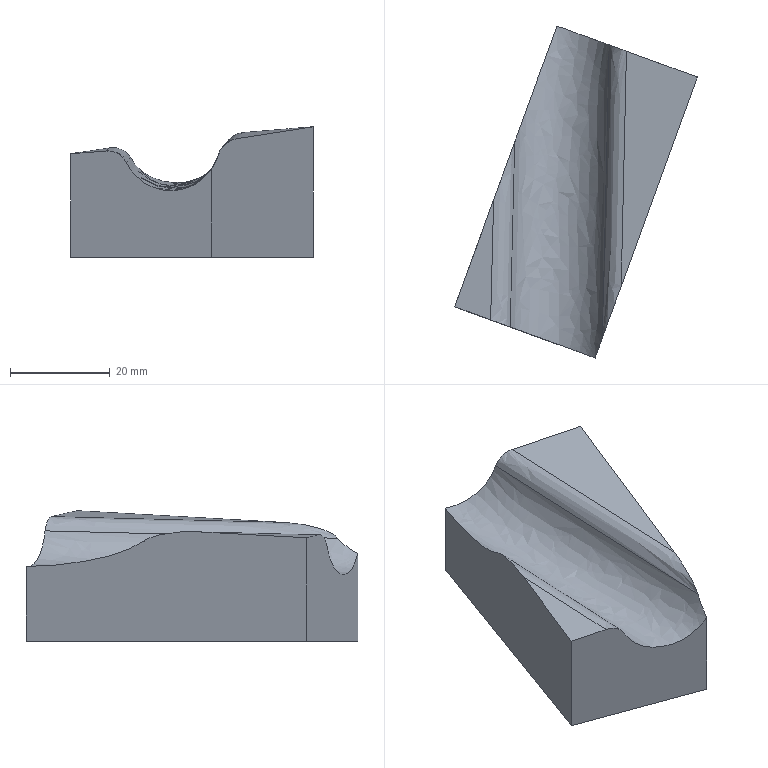Part | NX | features solid 2 | 1 solid | 10 faces | box 48.712 x 66.642 x 26.219 mm | volume 34058 mm3 | plane 5 | spline 5
STEP:
#1=CARTESIAN_POINT('',(673.941,90.778,15.));
#2=VERTEX_POINT('',#1);
#3=CARTESIAN_POINT('',(702.132,80.518,15.));
#4=VERTEX_POINT('',#3);
#5=CARTESIAN_POINT('',(673.941,90.778,15.));
#6=DIRECTION('',(-0.9397,0.342,0.));
#7=VECTOR('',#6,1000.);
#8=LINE('',#5,#7);
#9=EDGE_CURVE('',#2,#4,#8,.F.);
#10=ORIENTED_EDGE('',*,*,#9,.F.);
#11=CARTESIAN_POINT('',(694.463,147.16,15.));
#12=VERTEX_POINT('',#11);
#13=CARTESIAN_POINT('',(694.463,147.16,15.));
#14=DIRECTION('',(0.342,0.9397,0.));
#15=VECTOR('',#14,1000.);
#16=LINE('',#13,#15);
#17=EDGE_CURVE('',#12,#2,#16,.F.);
#18=ORIENTED_EDGE('',*,*,#17,.F.);
#19=CARTESIAN_POINT('',(722.653,136.899,15.));
#20=VERTEX_POINT('',#19);
#21=CARTESIAN_POINT('',(694.463,147.16,15.));
#22=DIRECTION('',(0.9397,-0.342,0.));
#23=VECTOR('',#22,1000.);
#24=LINE('',#21,#23);
#25=EDGE_CURVE('',#12,#20,#24,.T.);
#26=ORIENTED_EDGE('',*,*,#25,.T.);
#27=CARTESIAN_POINT('',(722.653,136.899,15.));
#28=DIRECTION('',(-0.342,-0.9397,0.));
#29=VECTOR('',#28,1000.);
#30=LINE('',#27,#29);
#31=EDGE_CURVE('',#20,#4,#30,.T.);
#32=ORIENTED_EDGE('',*,*,#31,.T.);
#33=EDGE_LOOP('',(#10,#18,#26,#32));
#34=FACE_BOUND('',#33,.T.);
#35=CARTESIAN_POINT('',(694.463,147.16,15.));
#36=DIRECTION('',(0.,0.,-1.));
#37=DIRECTION('',(-1.,0.,0.));
#38=AXIS2_PLACEMENT_3D('',#35,#36,#37);
#39=PLANE('',#38);
#40=ADVANCED_FACE('',(#34),#39,.T.);
#41=CARTESIAN_POINT('',(707.372,94.917,38.833));
#42=VERTEX_POINT('',#41);
#43=CARTESIAN_POINT('',(722.653,136.899,41.219));
#44=VERTEX_POINT('',#43);
#45=CARTESIAN_POINT('',(707.373,94.917,38.833));
#46=CARTESIAN_POINT('',(712.467,108.911,39.622));
#47=CARTESIAN_POINT('',(717.56,122.905,40.417));
#48=CARTESIAN_POINT('',(722.653,136.899,41.219));
#49=B_SPLINE_CURVE_WITH_KNOTS('',3,(#45,#46,#47,#48),.UNSPECIFIED.,.F.,.F.,(4,4),(0.01534,0.06009),.UNSPECIFIED.);
#50=EDGE_CURVE('',#42,#44,#49,.T.);
#51=ORIENTED_EDGE('',*,*,#50,.F.);
#52=CARTESIAN_POINT('',(703.614,84.589,35.684));
#53=VERTEX_POINT('',#52);
#54=CARTESIAN_POINT('',(707.373,94.917,38.833));
#55=CARTESIAN_POINT('',(707.041,94.005,38.782));
#56=CARTESIAN_POINT('',(706.382,92.195,38.607));
#57=CARTESIAN_POINT('',(705.407,89.515,38.119));
#58=CARTESIAN_POINT('',(704.453,86.895,37.295));
#59=CARTESIAN_POINT('',(703.838,85.206,36.423));
#60=CARTESIAN_POINT('',(703.614,84.59,35.686));
#61=B_SPLINE_CURVE_WITH_KNOTS('',3,(#54,#55,#56,#57,#58,#59,#60),.UNSPECIFIED.,.F.,.F.,(4,1,1,1,4),(0.,0.002892,0.005784,0.008676,0.01157),.UNSPECIFIED.);
#62=EDGE_CURVE('',#42,#53,#61,.T.);
#63=ORIENTED_EDGE('',*,*,#62,.T.);
#64=CARTESIAN_POINT('',(702.132,80.518,32.614));
#65=VERTEX_POINT('',#64);
#66=CARTESIAN_POINT('',(703.613,84.588,35.683));
#67=CARTESIAN_POINT('',(703.208,83.472,34.348));
#68=CARTESIAN_POINT('',(702.681,82.026,33.406));
#69=CARTESIAN_POINT('',(702.132,80.518,32.614));
#70=B_SPLINE_CURVE_WITH_KNOTS('',3,(#66,#67,#68,#69),.UNSPECIFIED.,.F.,.F.,(4,4),(0.0005394,0.005844),.UNSPECIFIED.);
#71=EDGE_CURVE('',#53,#65,#70,.T.);
#72=ORIENTED_EDGE('',*,*,#71,.T.);
#73=CARTESIAN_POINT('',(702.132,80.518,13.));
#74=DIRECTION('',(0.,0.,1.));
#75=VECTOR('',#74,1000.);
#76=LINE('',#73,#75);
#77=EDGE_CURVE('',#4,#65,#76,.T.);
#78=ORIENTED_EDGE('',*,*,#77,.F.);
#79=ORIENTED_EDGE('',*,*,#31,.F.);
#80=CARTESIAN_POINT('',(722.653,136.899,13.));
#81=DIRECTION('',(0.,0.,1.));
#82=VECTOR('',#81,1000.);
#83=LINE('',#80,#82);
#84=EDGE_CURVE('',#20,#44,#83,.T.);
#85=ORIENTED_EDGE('',*,*,#84,.T.);
#86=EDGE_LOOP('',(#51,#63,#72,#78,#79,#85));
#87=FACE_BOUND('',#86,.T.);
#88=CARTESIAN_POINT('',(722.653,136.899,13.));
#89=DIRECTION('',(0.9397,-0.342,0.));
#90=DIRECTION('',(-0.342,-0.9397,0.));
#91=AXIS2_PLACEMENT_3D('',#88,#89,#90);
#92=PLANE('',#91);
#93=ADVANCED_FACE('',(#87),#92,.T.);
#94=CARTESIAN_POINT('',(673.941,90.778,35.787));
#95=VERTEX_POINT('',#94);
#96=CARTESIAN_POINT('',(681.155,88.153,36.347));
#97=VERTEX_POINT('',#96);
#98=CARTESIAN_POINT('',(673.941,90.778,35.787));
#99=CARTESIAN_POINT('',(676.346,89.903,35.972));
#100=CARTESIAN_POINT('',(678.75,89.028,36.159));
#101=CARTESIAN_POINT('',(681.155,88.153,36.347));
#102=B_SPLINE_CURVE_WITH_KNOTS('',3,(#98,#99,#100,#101),.UNSPECIFIED.,.F.,.F.,(4,4),(0.,0.007697),.UNSPECIFIED.);
#103=EDGE_CURVE('',#95,#97,#102,.T.);
#104=ORIENTED_EDGE('',*,*,#103,.F.);
#105=CARTESIAN_POINT('',(673.941,90.778,13.));
#106=DIRECTION('',(0.,0.,1.));
#107=VECTOR('',#106,1000.);
#108=LINE('',#105,#107);
#109=EDGE_CURVE('',#2,#95,#108,.T.);
#110=ORIENTED_EDGE('',*,*,#109,.F.);
#111=ORIENTED_EDGE('',*,*,#9,.T.);
#112=ORIENTED_EDGE('',*,*,#77,.T.);
#113=CARTESIAN_POINT('',(685.071,86.728,34.051));
#114=VERTEX_POINT('',#113);
#115=CARTESIAN_POINT('',(702.132,80.518,32.614));
#116=CARTESIAN_POINT('',(700.144,81.242,29.648));
#117=CARTESIAN_POINT('',(693.105,83.803,26.583));
#118=CARTESIAN_POINT('',(686.604,86.17,30.796));
#119=CARTESIAN_POINT('',(685.071,86.728,34.051));
#120=B_SPLINE_CURVE_WITH_KNOTS('',3,(#115,#116,#117,#118,#119),.UNSPECIFIED.,.F.,.F.,(4,1,4),(0.,0.01075,0.0215),.UNSPECIFIED.);
#121=EDGE_CURVE('',#65,#114,#120,.T.);
#122=ORIENTED_EDGE('',*,*,#121,.T.);
#123=CARTESIAN_POINT('',(685.071,86.728,34.051));
#124=CARTESIAN_POINT('',(684.357,86.988,35.567));
#125=CARTESIAN_POINT('',(682.743,87.575,36.471));
#126=CARTESIAN_POINT('',(681.156,88.153,36.347));
#127=B_SPLINE_CURVE_WITH_KNOTS('',3,(#123,#124,#125,#126),.UNSPECIFIED.,.F.,.F.,(4,4),(0.,0.005011),.UNSPECIFIED.);
#128=EDGE_CURVE('',#114,#97,#127,.T.);
#129=ORIENTED_EDGE('',*,*,#128,.T.);
#130=EDGE_LOOP('',(#104,#110,#111,#112,#122,#129));
#131=FACE_BOUND('',#130,.T.);
#132=CARTESIAN_POINT('',(673.941,90.778,13.));
#133=DIRECTION('',(0.342,0.9397,0.));
#134=DIRECTION('',(0.9397,-0.342,0.));
#135=AXIS2_PLACEMENT_3D('',#132,#133,#134);
#136=PLANE('',#135);
#137=ADVANCED_FACE('',(#131),#136,.F.);
#138=CARTESIAN_POINT('',(681.758,112.256,36.959));
#139=VERTEX_POINT('',#138);
#140=CARTESIAN_POINT('',(681.758,112.256,36.959));
#141=CARTESIAN_POINT('',(679.153,105.097,36.567));
#142=CARTESIAN_POINT('',(676.547,97.938,36.176));
#143=CARTESIAN_POINT('',(673.941,90.778,35.787));
#144=B_SPLINE_CURVE_WITH_KNOTS('',3,(#140,#141,#142,#143),.UNSPECIFIED.,.F.,.F.,(4,4),(0.03719,0.06008),.UNSPECIFIED.);
#145=EDGE_CURVE('',#139,#95,#144,.T.);
#146=ORIENTED_EDGE('',*,*,#145,.F.);
#147=CARTESIAN_POINT('',(685.973,123.834,34.991));
#148=VERTEX_POINT('',#147);
#149=CARTESIAN_POINT('',(681.758,112.256,36.959));
#150=CARTESIAN_POINT('',(682.48,114.238,37.067));
#151=CARTESIAN_POINT('',(683.556,117.194,37.));
#152=CARTESIAN_POINT('',(684.984,121.118,36.247));
#153=CARTESIAN_POINT('',(685.663,122.984,35.579));
#154=CARTESIAN_POINT('',(685.973,123.834,34.991));
#155=B_SPLINE_CURVE_WITH_KNOTS('',3,(#149,#150,#151,#152,#153,#154),.UNSPECIFIED.,.F.,.F.,(4,1,1,4),(0.,0.006299,0.009448,0.0126),.UNSPECIFIED.);
#156=EDGE_CURVE('',#139,#148,#155,.T.);
#157=ORIENTED_EDGE('',*,*,#156,.T.);
#158=CARTESIAN_POINT('',(694.463,147.16,30.025));
#159=VERTEX_POINT('',#158);
#160=CARTESIAN_POINT('',(685.973,123.834,34.991));
#161=CARTESIAN_POINT('',(686.592,125.535,33.816));
#162=CARTESIAN_POINT('',(687.975,129.336,32.282));
#163=CARTESIAN_POINT('',(690.829,137.177,30.562));
#164=CARTESIAN_POINT('',(693.001,143.144,30.075));
#165=CARTESIAN_POINT('',(694.463,147.16,30.025));
#166=B_SPLINE_CURVE_WITH_KNOTS('',3,(#160,#161,#162,#163,#164,#165),.UNSPECIFIED.,.F.,.F.,(4,1,1,4),(0.000493,0.006904,0.01332,0.02614),.UNSPECIFIED.);
#167=EDGE_CURVE('',#148,#159,#166,.T.);
#168=ORIENTED_EDGE('',*,*,#167,.T.);
#169=CARTESIAN_POINT('',(694.463,147.16,13.));
#170=DIRECTION('',(0.,0.,1.));
#171=VECTOR('',#170,1000.);
#172=LINE('',#169,#171);
#173=EDGE_CURVE('',#12,#159,#172,.T.);
#174=ORIENTED_EDGE('',*,*,#173,.F.);
#175=ORIENTED_EDGE('',*,*,#17,.T.);
#176=ORIENTED_EDGE('',*,*,#109,.T.);
#177=EDGE_LOOP('',(#146,#157,#168,#174,#175,#176));
#178=FACE_BOUND('',#177,.T.);
#179=CARTESIAN_POINT('',(694.463,147.16,13.));
#180=DIRECTION('',(0.9397,-0.342,0.));
#181=DIRECTION('',(-0.342,-0.9397,0.));
#182=AXIS2_PLACEMENT_3D('',#179,#180,#181);
#183=PLANE('',#182);
#184=ADVANCED_FACE('',(#178),#183,.F.);
#185=CARTESIAN_POINT('',(708.428,142.077,40.024));
#186=VERTEX_POINT('',#185);
#187=CARTESIAN_POINT('',(722.653,136.899,41.219));
#188=CARTESIAN_POINT('',(717.911,138.625,40.815));
#189=CARTESIAN_POINT('',(713.168,140.352,40.416));
#190=CARTESIAN_POINT('',(708.425,142.078,40.024));
#191=B_SPLINE_CURVE_WITH_KNOTS('',3,(#187,#188,#189,#190),.UNSPECIFIED.,.F.,.F.,(4,4),(0.,0.01519),.UNSPECIFIED.);
#192=EDGE_CURVE('',#44,#186,#191,.T.);
#193=ORIENTED_EDGE('',*,*,#192,.F.);
#194=ORIENTED_EDGE('',*,*,#84,.F.);
#195=ORIENTED_EDGE('',*,*,#25,.F.);
#196=ORIENTED_EDGE('',*,*,#173,.T.);
#197=CARTESIAN_POINT('',(704.968,143.336,37.17));
#198=VERTEX_POINT('',#197);
#199=CARTESIAN_POINT('',(694.463,147.16,30.025));
#200=CARTESIAN_POINT('',(696.721,146.338,29.759));
#201=CARTESIAN_POINT('',(700.15,145.09,30.637));
#202=CARTESIAN_POINT('',(703.622,143.826,33.828));
#203=CARTESIAN_POINT('',(704.637,143.457,36.013));
#204=CARTESIAN_POINT('',(704.968,143.337,37.169));
#205=B_SPLINE_CURVE_WITH_KNOTS('',3,(#199,#200,#201,#202,#203,#204),.UNSPECIFIED.,.F.,.F.,(4,1,1,4),(0.,0.007147,0.01072,0.01429),.UNSPECIFIED.);
#206=EDGE_CURVE('',#159,#198,#205,.T.);
#207=ORIENTED_EDGE('',*,*,#206,.T.);
#208=CARTESIAN_POINT('',(704.969,143.336,37.172));
#209=CARTESIAN_POINT('',(705.423,143.171,38.764));
#210=CARTESIAN_POINT('',(706.872,142.643,39.895));
#211=CARTESIAN_POINT('',(708.429,142.077,40.024));
#212=B_SPLINE_CURVE_WITH_KNOTS('',3,(#208,#209,#210,#211),.UNSPECIFIED.,.F.,.F.,(4,4),(0.,0.004918),.UNSPECIFIED.);
#213=EDGE_CURVE('',#198,#186,#212,.T.);
#214=ORIENTED_EDGE('',*,*,#213,.T.);
#215=EDGE_LOOP('',(#193,#194,#195,#196,#207,#214));
#216=FACE_BOUND('',#215,.T.);
#217=CARTESIAN_POINT('',(694.463,147.16,13.));
#218=DIRECTION('',(0.342,0.9397,0.));
#219=DIRECTION('',(0.9397,-0.342,0.));
#220=AXIS2_PLACEMENT_3D('',#217,#218,#219);
#221=PLANE('',#220);
#222=ADVANCED_FACE('',(#216),#221,.T.);
#223=ORIENTED_EDGE('',*,*,#145,.T.);
#224=ORIENTED_EDGE('',*,*,#103,.T.);
#225=CARTESIAN_POINT('',(681.155,88.153,36.347));
#226=CARTESIAN_POINT('',(681.367,96.109,36.55));
#227=CARTESIAN_POINT('',(681.568,104.144,36.754));
#228=CARTESIAN_POINT('',(681.757,112.256,36.959));
#229=B_SPLINE_CURVE_WITH_KNOTS('',3,(#225,#226,#227,#228),.UNSPECIFIED.,.F.,.F.,(4,4),(0.786,0.8207),.UNSPECIFIED.);
#230=EDGE_CURVE('',#97,#139,#229,.T.);
#231=ORIENTED_EDGE('',*,*,#230,.T.);
#232=EDGE_LOOP('',(#223,#224,#231));
#233=FACE_BOUND('',#232,.T.);
#234=CARTESIAN_POINT('',(681.805,112.4,36.966));
#235=CARTESIAN_POINT('',(681.805,88.007,36.4));
#236=CARTESIAN_POINT('',(679.169,112.405,36.738));
#237=CARTESIAN_POINT('',(679.169,88.012,36.171));
#238=CARTESIAN_POINT('',(676.532,112.411,36.511));
#239=CARTESIAN_POINT('',(676.532,88.018,35.944));
#240=CARTESIAN_POINT('',(673.895,112.416,36.286));
#241=CARTESIAN_POINT('',(673.895,88.023,35.719));
#242=(BOUNDED_SURFACE()B_SPLINE_SURFACE(3,1,((#234,#235),(#236,#237),(#238,#239),(#240,#241)),.SURF_OF_LINEAR_EXTRUSION.,.F.,.F.,.F.)B_SPLINE_SURFACE_WITH_KNOTS((4,4),(2,2),(0.07819,0.08591),(0.3936,0.418),.PIECEWISE_BEZIER_KNOTS.)GEOMETRIC_REPRESENTATION_ITEM()RATIONAL_B_SPLINE_SURFACE(((0.9999,0.9999),(0.9999,0.9999),(0.9998,0.9998),(0.9998,0.9998)))REPRESENTATION_ITEM('')SURFACE());
#243=ADVANCED_FACE('',(#233),#242,.T.);
#244=ORIENTED_EDGE('',*,*,#167,.F.);
#245=CARTESIAN_POINT('',(685.973,123.834,34.991));
#246=CARTESIAN_POINT('',(685.712,111.846,34.69));
#247=CARTESIAN_POINT('',(685.414,99.477,34.377));
#248=CARTESIAN_POINT('',(685.071,86.728,34.051));
#249=B_SPLINE_CURVE_WITH_KNOTS('',3,(#245,#246,#247,#248),.UNSPECIFIED.,.F.,.F.,(4,4),(0.1752,0.2212),.UNSPECIFIED.);
#250=EDGE_CURVE('',#148,#114,#249,.T.);
#251=ORIENTED_EDGE('',*,*,#250,.T.);
#252=ORIENTED_EDGE('',*,*,#121,.F.);
#253=ORIENTED_EDGE('',*,*,#71,.F.);
#254=CARTESIAN_POINT('',(703.614,84.589,35.683));
#255=CARTESIAN_POINT('',(704.107,102.767,36.148));
#256=CARTESIAN_POINT('',(704.567,122.35,36.645));
#257=CARTESIAN_POINT('',(704.968,143.336,37.169));
#258=B_SPLINE_CURVE_WITH_KNOTS('',3,(#254,#255,#256,#257),.UNSPECIFIED.,.F.,.F.,(4,4),(0.7976,0.8799),.UNSPECIFIED.);
#259=EDGE_CURVE('',#53,#198,#258,.T.);
#260=ORIENTED_EDGE('',*,*,#259,.T.);
#261=ORIENTED_EDGE('',*,*,#206,.F.);
#262=EDGE_LOOP('',(#244,#251,#252,#253,#260,#261));
#263=FACE_BOUND('',#262,.T.);
#264=CARTESIAN_POINT('',(684.836,80.573,34.034));
#265=CARTESIAN_POINT('',(685.395,80.588,32.817));
#266=CARTESIAN_POINT('',(686.983,80.6,30.63));
#267=CARTESIAN_POINT('',(690.654,80.548,28.608));
#268=CARTESIAN_POINT('',(694.446,80.455,28.043));
#269=CARTESIAN_POINT('',(698.157,80.325,29.003));
#270=CARTESIAN_POINT('',(700.432,80.22,30.588));
#271=CARTESIAN_POINT('',(702.388,80.108,32.764));
#272=CARTESIAN_POINT('',(703.122,80.05,34.223));
#273=CARTESIAN_POINT('',(703.526,80.,35.703));
#274=CARTESIAN_POINT('',(685.461,102.899,34.601));
#275=CARTESIAN_POINT('',(686.02,102.916,33.385));
#276=CARTESIAN_POINT('',(687.61,102.932,31.198));
#277=CARTESIAN_POINT('',(691.283,102.892,29.18));
#278=CARTESIAN_POINT('',(695.076,102.812,28.618));
#279=CARTESIAN_POINT('',(698.786,102.695,29.58));
#280=CARTESIAN_POINT('',(701.06,102.597,31.168));
#281=CARTESIAN_POINT('',(703.015,102.493,33.345));
#282=CARTESIAN_POINT('',(703.749,102.438,34.805));
#283=CARTESIAN_POINT('',(704.151,102.39,36.285));
#284=CARTESIAN_POINT('',(685.975,125.23,35.159));
#285=CARTESIAN_POINT('',(686.535,125.248,33.943));
#286=CARTESIAN_POINT('',(688.126,125.269,31.758));
#287=CARTESIAN_POINT('',(691.8,125.241,29.742));
#288=CARTESIAN_POINT('',(695.594,125.173,29.183));
#289=CARTESIAN_POINT('',(699.304,125.069,30.148));
#290=CARTESIAN_POINT('',(701.577,124.98,31.737));
#291=CARTESIAN_POINT('',(703.531,124.883,33.916));
#292=CARTESIAN_POINT('',(704.264,124.83,35.376));
#293=CARTESIAN_POINT('',(704.666,124.784,36.857));
#294=CARTESIAN_POINT('',(686.392,147.565,35.71));
#295=CARTESIAN_POINT('',(686.953,147.585,34.495));
#296=CARTESIAN_POINT('',(688.545,147.61,32.31));
#297=CARTESIAN_POINT('',(692.22,147.593,30.297));
#298=CARTESIAN_POINT('',(696.015,147.537,29.739));
#299=CARTESIAN_POINT('',(699.725,147.444,30.707));
#300=CARTESIAN_POINT('',(701.997,147.363,32.297));
#301=CARTESIAN_POINT('',(703.95,147.273,34.477));
#302=CARTESIAN_POINT('',(704.682,147.223,35.938));
#303=CARTESIAN_POINT('',(705.083,147.179,37.419));
#304=B_SPLINE_SURFACE_WITH_KNOTS('',3,3,((#264,#265,#266,#267,#268,#269,#270,#271,#272,#273),(#274,#275,#276,#277,#278,#279,#280,#281,#282,#283),(#284,#285,#286,#287,#288,#289,#290,#291,#292,#293),(#294,#295,#296,#297,#298,#299,#300,#301,#302,#303)),.UNSPECIFIED.,.F.,.F.,.F.,(4,4),(4,1,1,1,1,2,4),(0.8164,0.8916),(0.1207,0.2428,0.3625,0.4822,0.6019,0.7216,0.8613),.UNSPECIFIED.);
#305=ADVANCED_FACE('',(#263),#304,.F.);
#306=ORIENTED_EDGE('',*,*,#230,.F.);
#307=ORIENTED_EDGE('',*,*,#128,.F.);
#308=ORIENTED_EDGE('',*,*,#250,.F.);
#309=ORIENTED_EDGE('',*,*,#156,.F.);
#310=EDGE_LOOP('',(#306,#307,#308,#309));
#311=FACE_BOUND('',#310,.T.);
#312=CARTESIAN_POINT('',(682.025,124.086,37.257));
#313=CARTESIAN_POINT('',(684.782,124.02,37.494));
#314=CARTESIAN_POINT('',(685.977,124.057,34.997));
#315=CARTESIAN_POINT('',(681.753,111.575,36.942));
#316=CARTESIAN_POINT('',(684.511,111.504,37.18));
#317=CARTESIAN_POINT('',(685.706,111.539,34.682));
#318=CARTESIAN_POINT('',(681.45,99.064,36.626));
#319=CARTESIAN_POINT('',(684.208,98.988,36.863));
#320=CARTESIAN_POINT('',(685.402,99.022,34.365));
#321=CARTESIAN_POINT('',(681.113,86.554,36.306));
#322=CARTESIAN_POINT('',(683.87,86.474,36.543));
#323=CARTESIAN_POINT('',(685.065,86.505,34.045));
#324=(BOUNDED_SURFACE()B_SPLINE_SURFACE(3,2,((#312,#313,#314),(#315,#316,#317),(#318,#319,#320),(#321,#322,#323)),.UNSPECIFIED.,.F.,.F.,.F.)B_SPLINE_SURFACE_WITH_KNOTS((4,4),(3,3),(0.6997,0.7373),(0.,1.),.PIECEWISE_BEZIER_KNOTS.)GEOMETRIC_REPRESENTATION_ITEM()RATIONAL_B_SPLINE_SURFACE(((1.,0.8222,1.),(1.,0.8222,1.),(1.,0.8222,1.),(1.,0.8222,1.)))REPRESENTATION_ITEM('')SURFACE());
#325=ADVANCED_FACE('',(#311),#324,.T.);
#326=ORIENTED_EDGE('',*,*,#259,.F.);
#327=ORIENTED_EDGE('',*,*,#62,.F.);
#328=CARTESIAN_POINT('',(708.425,142.077,40.024));
#329=CARTESIAN_POINT('',(708.118,126.077,39.624));
#330=CARTESIAN_POINT('',(707.766,110.357,39.227));
#331=CARTESIAN_POINT('',(707.371,94.917,38.833));
#332=B_SPLINE_CURVE_WITH_KNOTS('',3,(#328,#329,#330,#331),.UNSPECIFIED.,.F.,.F.,(4,4),(0.1291,0.1921),.UNSPECIFIED.);
#333=EDGE_CURVE('',#186,#42,#332,.T.);
#334=ORIENTED_EDGE('',*,*,#333,.F.);
#335=ORIENTED_EDGE('',*,*,#213,.F.);
#336=EDGE_LOOP('',(#326,#327,#334,#335));
#337=FACE_BOUND('',#336,.T.);
#338=CARTESIAN_POINT('',(704.975,143.689,37.181));
#339=CARTESIAN_POINT('',(705.729,143.609,39.813));
#340=CARTESIAN_POINT('',(708.457,143.551,40.061));
#341=CARTESIAN_POINT('',(704.598,123.869,36.687));
#342=CARTESIAN_POINT('',(705.352,123.786,39.319));
#343=CARTESIAN_POINT('',(708.079,123.721,39.566));
#344=CARTESIAN_POINT('',(704.144,104.051,36.186));
#345=CARTESIAN_POINT('',(704.899,103.966,38.818));
#346=CARTESIAN_POINT('',(707.626,103.893,39.064));
#347=CARTESIAN_POINT('',(703.605,84.237,35.677));
#348=CARTESIAN_POINT('',(704.359,84.148,38.309));
#349=CARTESIAN_POINT('',(707.086,84.068,38.555));
#350=(BOUNDED_SURFACE()B_SPLINE_SURFACE(3,2,((#338,#339,#340),(#341,#342,#343),(#344,#345,#346),(#347,#348,#349)),.UNSPECIFIED.,.F.,.F.,.F.)B_SPLINE_SURFACE_WITH_KNOTS((4,4),(3,3),(0.6753,0.7349),(0.,1.),.PIECEWISE_BEZIER_KNOTS.)GEOMETRIC_REPRESENTATION_ITEM()RATIONAL_B_SPLINE_SURFACE(((1.,0.8251,1.),(1.,0.8251,1.),(1.,0.8251,1.),(1.,0.8251,1.)))REPRESENTATION_ITEM('')SURFACE());
#351=ADVANCED_FACE('',(#337),#350,.T.);
#352=ORIENTED_EDGE('',*,*,#192,.T.);
#353=ORIENTED_EDGE('',*,*,#333,.T.);
#354=ORIENTED_EDGE('',*,*,#50,.T.);
#355=EDGE_LOOP('',(#352,#353,#354));
#356=FACE_BOUND('',#355,.T.);
#357=CARTESIAN_POINT('',(722.745,142.33,41.353));
#358=CARTESIAN_POINT('',(722.745,94.601,40.245));
#359=CARTESIAN_POINT('',(717.591,142.341,40.871));
#360=CARTESIAN_POINT('',(717.591,94.612,39.763));
#361=CARTESIAN_POINT('',(712.435,142.353,40.395));
#362=CARTESIAN_POINT('',(712.435,94.623,39.287));
#363=CARTESIAN_POINT('',(707.28,142.363,39.926));
#364=CARTESIAN_POINT('',(707.28,94.634,38.818));
#365=(BOUNDED_SURFACE()B_SPLINE_SURFACE(3,1,((#357,#358),(#359,#360),(#361,#362),(#363,#364)),.SURF_OF_LINEAR_EXTRUSION.,.F.,.F.,.F.)B_SPLINE_SURFACE_WITH_KNOTS((4,4),(2,2),(0.03822,0.05333),(0.3637,0.4113),.PIECEWISE_BEZIER_KNOTS.)GEOMETRIC_REPRESENTATION_ITEM()RATIONAL_B_SPLINE_SURFACE(((0.9999,0.9999),(0.9999,0.9999),(0.9999,0.9999),(0.9999,0.9999)))REPRESENTATION_ITEM('')SURFACE());
#366=ADVANCED_FACE('',(#356),#365,.T.);
#367=CLOSED_SHELL('',(#40,#93,#137,#184,#222,#243,#305,#325,#351,#366));
#368=MANIFOLD_SOLID_BREP('',#367);
#369=(LENGTH_UNIT()NAMED_UNIT(*)SI_UNIT(.MILLI.,.METRE.));
#370=UNCERTAINTY_MEASURE_WITH_UNIT(LENGTH_MEASURE(0.05706),#369,'','');
#371=(NAMED_UNIT(*)PLANE_ANGLE_UNIT()SI_UNIT($,.RADIAN.));
#372=(NAMED_UNIT(*)SI_UNIT($,.STERADIAN.)SOLID_ANGLE_UNIT());
#373=(GEOMETRIC_REPRESENTATION_CONTEXT(3)GLOBAL_UNCERTAINTY_ASSIGNED_CONTEXT((#370))GLOBAL_UNIT_ASSIGNED_CONTEXT((#369,#371,#372))REPRESENTATION_CONTEXT('',''));
#374=ADVANCED_BREP_SHAPE_REPRESENTATION('',(#368),#373);